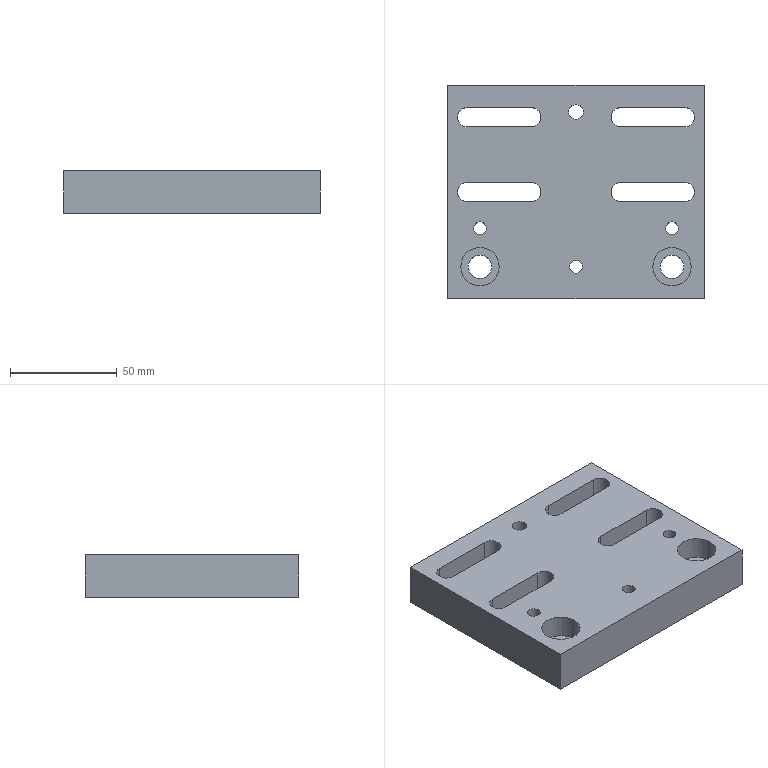CAM job | NX | 3-axis milling, drilling | part box 120 x 100 x 20 mm | stock box 125 x 100 x 25 mm
Tools:
number,name,description,diameter,corner_radius,flute_length,length,flutes
6,D6,平底铣刀-粗,6.0,0.0,25.0,75.0,2
9,D10,平底铣刀-粗,10.0,0.0,35.0,75.0,2
7,D6-J,平底铣刀-精,6.0,0.0,25.0,75.0,2
10,D10-J,平底铣刀-精,10.0,0.0,35.0,75.0,2
1,D80R0.8飞刀,圆鼻刀-粗,80.0,0.8,50.0,75.0,2
1,D80R0.8飞刀-J,圆鼻刀-精,80.0,0.8,50.0,75.0,2
2,D6倒角刀,倒角刀,6.0,0.0,3.0,25.0,2
22,M8X1.25,丝锥,6.8,0.0,35.0,50.0,2
19,D6铰刀,Drilling Tool,6.0,0.0,75.0,100.0,6
18,ZT11,钻头,11.0,0.0,35.0,50.0,2
17,ZT5.9,Drilling Tool,5.9,0.0,35.0,50.0,2
16,ZT6.9,Drilling Tool,6.9,0.0,35.0,50.0,2
Operations:
program,operation,operation_type,tool,method,geometry_group,spindle_rpm,surface_speed,feed_per_tooth,feed_cut,feed_plunge,cut_length_mm,path_length_mm,cut_time_min,machine_time_min
B,BOTTOMWALL_FLYCUT_ROUGH_COPY,VolumeBased25DMillingOperation,D80R0.8飞刀,ZLEVEL_ROUGH_DEPTHK_STEPG,W-B,2800.0,703.696,0.5357,3000.0,100.0,4200.277,4650.855,1.4,1.445
B,BOTTOMWALL_FLYCUT_FINISH_COPY,VolumeBased25DMillingOperation,D80R0.8飞刀-J,SIDEFINISH_DEPTHK_STEPG,W-B,4000.0,1005.28,0.125,1000.0,100.0,466.11,562.11,0.4661,0.4757
B,CHAMFER_MILL_4,PlanarMilling,D6倒角刀,METHOD,W-B,8000.0,150.796,0.0375,600.0,100.0,56.866,459.253,0.0948,0.135
B,CHAMFER_MILL_5,PlanarMilling,D6倒角刀,METHOD,W-B,8000.0,150.796,0.0375,600.0,100.0,31.274,133.074,0.0521,0.0623
B,CHAMFER_MILL_6,PlanarMilling,D6倒角刀,METHOD,W-B,8000.0,150.796,0.075,1200.0,100.0,66.997,364.332,0.0558,0.0856
B,PLANARDEBURR_6X45L_COPY,SurfaceContour,D6倒角刀,CLIMBCHAMFER_DEPTH0_STEPG,W-B,6500.0,122.519,0.1154,1500.0,100.0,924.623,1577.348,0.6164,0.6817
A,TOPFACE,FaceMilling,D80R0.8飞刀,SIDEFINISH_DEPTHK_STEPG,W-A,4500.0,1385.0,0.1667,1500.0,100.0,704.0,800.0,0.4693,0.4789
A,PROFILE_ROUGH_2,VolumeBased25DMillingOperation,D10,METHOD,W-A,8000.0,251.327,0.375,6000.0,80.0,12746.712,12865.212,2.124,2.136
A,SPOTDRILL_DEPTH0.8,Operation,D6倒角刀,NONE,W-A,8000.0,150.796,0.0312,500.0,90.0,10.8,323.362,0.0216,0.0529
A,THRUHOLE_REAMPILOT6.0,Operation,ZT5.9,NONE,W-A,2500.0,46.339,0.05,250.0,90.0,77.109,353.173,0.3084,0.336
A,THRUHOLE_M8TAPDRILL,Operation,ZT6.9,NONE,W-A,1800.0,38.453,0.0972,350.0,90.0,30.0,160.0,0.0857,0.0987
A,COUNTERBORE_DRILL_SEG0,Operation,ZT11,NONE,W-A,800.0,27.646,0.0938,150.0,90.0,52.609,296.224,0.3507,0.3751
A,THRUSLOT_ROUGH_1,VolumeBased25DMillingOperation,D6,METHOD,W-A,9000.0,169.646,0.1389,2500.0,100.0,11564.103,12179.61,4.626,4.687
A,HOLE_ROUGH_D8_1,CylinderMilling,D10,NONE,W-A,8000.0,201.062,0.075,1200.0,100.0,1161.736,1471.936,0.9681,0.9991
A,HOLE_FINISH_D8_1,CylinderMilling,D10-J,FINISHSTEPDEPTHOFF,W-A,8000.0,201.062,0.0312,500.0,100.0,188.14,498.34,0.3763,0.4073
A,SLOT_FINISH_1,VolumeBased25DMillingOperation,D6-J,METHOD,W-A,8000.0,150.796,0.0375,600.0,100.0,1146.449,1986.373,1.911,1.995
A,BODYONLY,SurfaceContour,D6倒角刀,METHOD,W-A,8000.0,150.796,0.1875,3000.0,100.0,929.471,1920.579,0.3098,0.4089
A,CHAMFER_MILL_1,PlanarMilling,D6倒角刀,METHOD,W-A,8000.0,150.796,0.0312,500.0,100.0,62.891,462.918,0.1258,0.1658
A,CHAMFER_MILL_2,PlanarMilling,D6倒角刀,METHOD,W-A,8000.0,150.796,0.0375,600.0,100.0,24.401,126.001,0.0407,0.0508
A,CHAMFER_MILL_3,PlanarMilling,D6倒角刀,NONE,W-A,8000.0,150.796,0.05,800.0,100.0,130.768,408.195,0.1635,0.1912
A,REAMING,Operation,D6铰刀,METHOD,W-A,500.0,9.425,0.0167,50.0,0.0,66.0,330.954,1.32,1.347
A,THRUHOLE_TAPM8,Operation,M8X1.25,METHOD,W-A,500.0,10.681,0.0013,1.25,90.0,25.0,150.0,20.0,20.012
A,PROFILE_SEMIFINISH_2,VolumeBased25DMillingOperation,D10-J,METHOD,W-A,9000.0,169.646,0.0667,1200.0,100.0,952.748,1213.263,0.794,0.82
A,BOTTOMWALL_SIDEFINISH_MID_COPY,VolumeBased25DMillingOperation,D10-J,SIDEFINISH_DEPTHK_STEPG,W-A,8000.0,251.32,0.0625,1000.0,100.0,550.256,1025.85,0.5503,0.5978